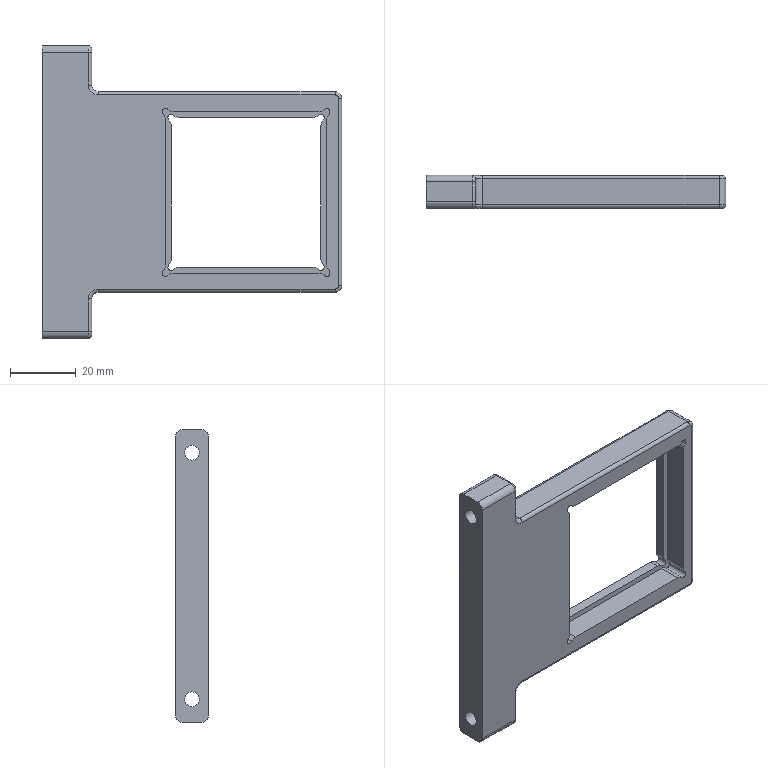NC program | NX | posted by the shop | part box 91 x 10 x 89 mm
Lines 7061 to 8910 of 16928, first 1495 of 1850 lines:
N4 T11 M06
(D4-J  D=4. R=0. H=11 ce=0.00 di=0.01)
G00 G90 G54 X-24.947 Y-33.1 M03 S9000
G43 H11 Z20.
M08
Z-.571
G01 X-24.948 Y-33.094 Z-.656 F2000.
X-24.951 Y-33.074 Z-.734
X-24.956 Y-33.045 Z-.804
X-24.964 Y-33.006 Z-.867
X-24.975 Y-32.961 Z-.922
X-24.989 Y-32.91 Z-.971
X-25.006 Y-32.856 Z-1.014
X-25.027 Y-32.8 Z-1.051
X-25.051 Y-32.744 Z-1.082
X-25.08 Y-32.69 Z-1.107
X-25.112 Y-32.639 Z-1.128
X-25.149 Y-32.594 Z-1.144
X-25.191 Y-32.555 Z-1.156
X-25.238 Y-32.526 Z-1.164
X-25.29 Y-32.507 Z-1.169
X-25.347 Y-32.5 Z-1.171
X-28.489 F2500.
X-28.5
Y-35.653
X-28.484 Y-35.696
X-28.438 Y-35.718 Z-1.174
X-28.366 Y-35.719 Z-1.178
X-28.271 Y-35.702 Z-1.184
X-28.156 Y-35.669 Z-1.19
X-28.026 Y-35.62 Z-1.198
X-27.882 Y-35.557 Z-1.207
X-27.73 Y-35.483 Z-1.217
X-27.571 Y-35.398 Z-1.227
X-27.41 Y-35.304 Z-1.238
X-27.25 Y-35.203 Z-1.25
X-26.913 Y-34.962 Z-1.276
X-26.597 Y-34.695 Z-1.303
X-26.306 Y-34.403 Z-1.331
X-26.038 Y-34.088 Z-1.358
X-25.797 Y-33.75 Z-1.384
X-25.696 Y-33.59 Z-1.395
X-25.602 Y-33.429 Z-1.406
X-25.517 Y-33.27 Z-1.417
X-25.443 Y-33.118 Z-1.427
X-25.38 Y-32.974 Z-1.436
X-25.331 Y-32.844 Z-1.443
X-25.298 Y-32.729 Z-1.45
X-25.281 Y-32.634 Z-1.456
X-25.282 Y-32.562 Z-1.46
X-25.304 Y-32.516 Z-1.462
X-25.347 Y-32.5 Z-1.463
X-28.489
X-28.5
Y-35.653
X-28.484 Y-35.696 Z-1.464
X-28.438 Y-35.718 Z-1.467
X-28.366 Y-35.719 Z-1.471
X-28.271 Y-35.702 Z-1.476
X-28.156 Y-35.669 Z-1.483
X-28.026 Y-35.62 Z-1.491
X-27.882 Y-35.557 Z-1.5
X-27.73 Y-35.483 Z-1.51
X-27.571 Y-35.398 Z-1.52
X-27.41 Y-35.304 Z-1.531
X-27.25 Y-35.203 Z-1.542
X-26.913 Y-34.962 Z-1.569
X-26.597 Y-34.695 Z-1.596
X-26.306 Y-34.403 Z-1.623
X-26.038 Y-34.088 Z-1.65
X-25.797 Y-33.75 Z-1.677
X-25.696 Y-33.59 Z-1.688
X-25.602 Y-33.429 Z-1.699
X-25.517 Y-33.27 Z-1.71
X-25.443 Y-33.118 Z-1.719
X-25.38 Y-32.974 Z-1.728
X-25.331 Y-32.844 Z-1.736
X-25.298 Y-32.729 Z-1.743
X-25.281 Y-32.634 Z-1.748
X-25.282 Y-32.562 Z-1.752
X-25.304 Y-32.516 Z-1.755
X-25.347 Y-32.5 Z-1.756
X-28.489
X-28.5
Y-35.653
X-28.484 Y-35.696 Z-1.757
X-28.438 Y-35.718 Z-1.759
X-28.366 Y-35.719 Z-1.763
X-28.271 Y-35.702 Z-1.769
X-28.156 Y-35.669 Z-1.776
X-28.026 Y-35.62 Z-1.784
X-27.882 Y-35.557 Z-1.792
X-27.73 Y-35.483 Z-1.802
X-27.571 Y-35.398 Z-1.813
X-27.41 Y-35.304 Z-1.824
X-27.25 Y-35.203 Z-1.835
X-26.913 Y-34.962 Z-1.861
X-26.597 Y-34.695 Z-1.889
X-26.306 Y-34.403 Z-1.916
X-26.038 Y-34.088 Z-1.943
X-25.797 Y-33.75 Z-1.969
X-25.696 Y-33.59 Z-1.981
X-25.602 Y-33.429 Z-1.992
X-25.517 Y-33.27 Z-2.002
X-25.443 Y-33.118 Z-2.012
X-25.38 Y-32.974 Z-2.021
X-25.331 Y-32.844 Z-2.029
X-25.298 Y-32.729 Z-2.035
X-25.281 Y-32.634 Z-2.041
X-25.282 Y-32.562 Z-2.045
X-25.304 Y-32.516 Z-2.048
X-25.347 Y-32.5 Z-2.049
X-28.489
X-28.5
Y-35.653
X-28.484 Y-35.696
X-28.438 Y-35.718 Z-2.052
X-28.366 Y-35.719 Z-2.056
X-28.271 Y-35.702 Z-2.062
X-28.156 Y-35.669 Z-2.068
X-28.026 Y-35.62 Z-2.076
X-27.882 Y-35.557 Z-2.085
X-27.73 Y-35.483 Z-2.095
X-27.571 Y-35.398 Z-2.105
X-27.41 Y-35.304 Z-2.116
X-27.25 Y-35.203 Z-2.128
X-26.913 Y-34.962 Z-2.154
X-26.597 Y-34.695 Z-2.181
X-26.306 Y-34.403 Z-2.209
X-26.038 Y-34.088 Z-2.236
X-25.797 Y-33.75 Z-2.262
X-25.696 Y-33.59 Z-2.273
X-25.602 Y-33.429 Z-2.284
X-25.517 Y-33.27 Z-2.295
X-25.443 Y-33.118 Z-2.305
X-25.38 Y-32.974 Z-2.313
X-25.331 Y-32.844 Z-2.321
X-25.298 Y-32.729 Z-2.328
X-25.281 Y-32.634 Z-2.334
X-25.282 Y-32.562 Z-2.338
X-25.304 Y-32.516 Z-2.34
X-25.347 Y-32.5 Z-2.341
X-28.489
X-28.5
Y-35.653
X-28.484 Y-35.696 Z-2.342
X-28.438 Y-35.718 Z-2.345
X-28.366 Y-35.719 Z-2.349
X-28.271 Y-35.702 Z-2.354
X-28.156 Y-35.669 Z-2.361
X-28.026 Y-35.62 Z-2.369
X-27.882 Y-35.557 Z-2.378
X-27.73 Y-35.483 Z-2.387
X-27.571 Y-35.398 Z-2.398
X-27.41 Y-35.304 Z-2.409
X-27.25 Y-35.203 Z-2.42
X-26.913 Y-34.962 Z-2.447
X-26.597 Y-34.695 Z-2.474
X-26.306 Y-34.403 Z-2.501
X-26.038 Y-34.088 Z-2.528
X-25.797 Y-33.75 Z-2.555
X-25.696 Y-33.59 Z-2.566
X-25.602 Y-33.429 Z-2.577
X-25.517 Y-33.27 Z-2.588
X-25.443 Y-33.118 Z-2.597
X-25.38 Y-32.974 Z-2.606
X-25.331 Y-32.844 Z-2.614
X-25.298 Y-32.729 Z-2.621
X-25.281 Y-32.634 Z-2.626
X-25.282 Y-32.562 Z-2.63
X-25.304 Y-32.516 Z-2.633
X-25.347 Y-32.5 Z-2.634
X-28.489
X-28.5
Y-35.653
X-28.484 Y-35.696 Z-2.635
X-28.438 Y-35.718 Z-2.637
X-28.366 Y-35.719 Z-2.641
X-28.271 Y-35.702 Z-2.647
X-28.156 Y-35.669 Z-2.654
X-28.026 Y-35.62 Z-2.662
X-27.882 Y-35.557 Z-2.67
X-27.73 Y-35.483 Z-2.68
X-27.571 Y-35.398 Z-2.691
X-27.41 Y-35.304 Z-2.702
X-27.25 Y-35.203 Z-2.713
X-26.913 Y-34.962 Z-2.739
X-26.597 Y-34.695 Z-2.766
X-26.306 Y-34.403 Z-2.794
X-26.038 Y-34.088 Z-2.821
X-25.797 Y-33.75 Z-2.847
X-25.696 Y-33.59 Z-2.859
X-25.602 Y-33.429 Z-2.87
X-25.517 Y-33.27 Z-2.88
X-25.443 Y-33.118 Z-2.89
X-25.38 Y-32.974 Z-2.899
X-25.331 Y-32.844 Z-2.907
X-25.298 Y-32.729 Z-2.913
X-25.281 Y-32.634 Z-2.919
X-25.282 Y-32.562 Z-2.923
X-25.304 Y-32.516 Z-2.926
X-25.347 Y-32.5
X-28.489
X-28.5
Y-35.653
X-28.484 Y-35.696 Z-2.927
X-28.438 Y-35.718 Z-2.93
X-28.366 Y-35.719 Z-2.934
X-28.271 Y-35.702 Z-2.94
X-28.156 Y-35.669 Z-2.946
X-28.026 Y-35.62 Z-2.954
X-27.882 Y-35.557 Z-2.963
X-27.73 Y-35.483 Z-2.973
X-27.571 Y-35.398 Z-2.983
X-27.41 Y-35.304 Z-2.994
X-27.25 Y-35.203 Z-3.006
X-26.913 Y-34.962 Z-3.032
X-26.597 Y-34.695 Z-3.059
X-26.306 Y-34.403 Z-3.087
X-26.038 Y-34.088 Z-3.114
X-25.797 Y-33.75 Z-3.14
X-25.696 Y-33.59 Z-3.151
X-25.602 Y-33.429 Z-3.162
X-25.517 Y-33.27 Z-3.173
X-25.443 Y-33.118 Z-3.183
X-25.38 Y-32.974 Z-3.191
X-25.331 Y-32.844 Z-3.199
X-25.298 Y-32.729 Z-3.206
X-25.281 Y-32.634 Z-3.212
X-25.282 Y-32.562 Z-3.216
X-25.304 Y-32.516 Z-3.218
X-25.347 Y-32.5 Z-3.219
X-28.489
X-28.5
Y-35.653
X-28.484 Y-35.696 Z-3.22
X-28.438 Y-35.718 Z-3.223
X-28.366 Y-35.719 Z-3.227
X-28.271 Y-35.702 Z-3.232
X-28.156 Y-35.669 Z-3.239
X-28.026 Y-35.62 Z-3.247
X-27.882 Y-35.557 Z-3.256
X-27.73 Y-35.483 Z-3.265
X-27.571 Y-35.398 Z-3.276
X-27.41 Y-35.304 Z-3.287
X-27.25 Y-35.203 Z-3.298
X-26.913 Y-34.962 Z-3.325
X-26.597 Y-34.695 Z-3.352
X-26.306 Y-34.403 Z-3.379
X-26.038 Y-34.088 Z-3.406
X-25.797 Y-33.75 Z-3.433
X-25.696 Y-33.59 Z-3.444
X-25.602 Y-33.429 Z-3.455
X-25.517 Y-33.27 Z-3.465
X-25.443 Y-33.118 Z-3.475
X-25.38 Y-32.974 Z-3.484
X-25.331 Y-32.844 Z-3.492
X-25.298 Y-32.729 Z-3.499
X-25.281 Y-32.634 Z-3.504
X-25.282 Y-32.562 Z-3.508
X-25.304 Y-32.516 Z-3.511
X-25.347 Y-32.5 Z-3.512
X-28.489
X-28.5
Y-35.653
X-28.484 Y-35.696 Z-3.513
X-28.438 Y-35.718 Z-3.515
X-28.366 Y-35.719 Z-3.519
X-28.271 Y-35.702 Z-3.525
X-28.156 Y-35.669 Z-3.532
X-28.026 Y-35.62 Z-3.539
X-27.882 Y-35.557 Z-3.548
X-27.73 Y-35.483 Z-3.558
X-27.571 Y-35.398 Z-3.569
X-27.41 Y-35.304 Z-3.58
X-27.25 Y-35.203 Z-3.591
X-26.913 Y-34.962 Z-3.617
X-26.597 Y-34.695 Z-3.644
X-26.306 Y-34.403 Z-3.672
X-26.038 Y-34.088 Z-3.699
X-25.797 Y-33.75 Z-3.725
X-25.696 Y-33.59 Z-3.737
X-25.602 Y-33.429 Z-3.748
X-25.517 Y-33.27 Z-3.758
X-25.443 Y-33.118 Z-3.768
X-25.38 Y-32.974 Z-3.777
X-25.331 Y-32.844 Z-3.785
X-25.298 Y-32.729 Z-3.791
X-25.281 Y-32.634 Z-3.797
X-25.282 Y-32.562 Z-3.801
X-25.304 Y-32.516 Z-3.804
X-25.347 Y-32.5
X-28.489
X-28.5
Y-35.653
X-28.484 Y-35.696 Z-3.805
X-28.438 Y-35.718 Z-3.808
X-28.366 Y-35.719 Z-3.812
X-28.271 Y-35.702 Z-3.817
X-28.156 Y-35.669 Z-3.824
X-28.026 Y-35.62 Z-3.832
X-27.882 Y-35.557 Z-3.841
X-27.73 Y-35.483 Z-3.851
X-27.571 Y-35.398 Z-3.861
X-27.41 Y-35.304 Z-3.872
X-27.25 Y-35.203 Z-3.884
X-26.913 Y-34.962 Z-3.91
X-26.597 Y-34.695 Z-3.937
X-26.306 Y-34.403 Z-3.964
X-26.038 Y-34.088 Z-3.992
X-25.797 Y-33.75 Z-4.018
X-25.696 Y-33.59 Z-4.029
X-25.602 Y-33.429 Z-4.04
X-25.517 Y-33.27 Z-4.051
X-25.443 Y-33.118 Z-4.06
X-25.38 Y-32.974 Z-4.069
X-25.331 Y-32.844 Z-4.077
X-25.298 Y-32.729 Z-4.084
X-25.281 Y-32.634 Z-4.09
X-25.282 Y-32.562 Z-4.094
X-25.304 Y-32.516 Z-4.096
X-25.347 Y-32.5 Z-4.097
X-28.489
X-28.5
Y-35.653
X-28.484 Y-35.696 Z-4.098
X-28.438 Y-35.718 Z-4.101
X-28.366 Y-35.719 Z-4.105
X-28.271 Y-35.702 Z-4.11
X-28.156 Y-35.669 Z-4.117
X-28.026 Y-35.62 Z-4.125
X-27.882 Y-35.557 Z-4.134
X-27.73 Y-35.483 Z-4.143
X-27.571 Y-35.398 Z-4.154
X-27.41 Y-35.304 Z-4.165
X-27.25 Y-35.203 Z-4.176
X-26.913 Y-34.962 Z-4.203
X-26.597 Y-34.695 Z-4.23
X-26.306 Y-34.403 Z-4.257
X-26.038 Y-34.088 Z-4.284
X-25.797 Y-33.75 Z-4.31
X-25.696 Y-33.59 Z-4.322
X-25.602 Y-33.429 Z-4.333
X-25.517 Y-33.27 Z-4.343
X-25.443 Y-33.118 Z-4.353
X-25.38 Y-32.974 Z-4.362
X-25.331 Y-32.844 Z-4.37
X-25.298 Y-32.729 Z-4.377
X-25.281 Y-32.634 Z-4.382
X-25.282 Y-32.562 Z-4.386
X-25.304 Y-32.516 Z-4.389
X-25.347 Y-32.5 Z-4.39
X-28.489
X-28.5
Y-35.653
X-28.484 Y-35.696 Z-4.391
X-28.438 Y-35.718 Z-4.393
X-28.366 Y-35.719 Z-4.397
X-28.271 Y-35.702 Z-4.403
X-28.156 Y-35.669 Z-4.41
X-28.026 Y-35.62 Z-4.417
X-27.882 Y-35.557 Z-4.426
X-27.73 Y-35.483 Z-4.436
X-27.571 Y-35.398 Z-4.446
X-27.41 Y-35.304 Z-4.458
X-27.25 Y-35.203 Z-4.469
X-26.913 Y-34.962 Z-4.495
X-26.597 Y-34.695 Z-4.522
X-26.306 Y-34.403 Z-4.55
X-26.038 Y-34.088 Z-4.577
X-25.797 Y-33.75 Z-4.603
X-25.696 Y-33.59 Z-4.615
X-25.602 Y-33.429 Z-4.626
X-25.517 Y-33.27 Z-4.636
X-25.443 Y-33.118 Z-4.646
X-25.38 Y-32.974 Z-4.655
X-25.331 Y-32.844 Z-4.663
X-25.298 Y-32.729 Z-4.669
X-25.281 Y-32.634 Z-4.675
X-25.282 Y-32.562 Z-4.679
X-25.304 Y-32.516 Z-4.681
X-25.347 Y-32.5 Z-4.682
X-28.489
X-28.5
Y-35.653
X-28.484 Y-35.696 Z-4.683
X-28.438 Y-35.718 Z-4.686
X-28.366 Y-35.719 Z-4.69
X-28.271 Y-35.702 Z-4.695
X-28.156 Y-35.669 Z-4.702
X-28.026 Y-35.62 Z-4.71
X-27.882 Y-35.557 Z-4.719
X-27.73 Y-35.483 Z-4.729
X-27.571 Y-35.398 Z-4.739
X-27.41 Y-35.304 Z-4.75
X-27.25 Y-35.203 Z-4.762
X-26.913 Y-34.962 Z-4.788
X-26.597 Y-34.695 Z-4.815
X-26.306 Y-34.403 Z-4.842
X-26.038 Y-34.088 Z-4.87
X-25.797 Y-33.75 Z-4.896
X-25.696 Y-33.59 Z-4.907
X-25.602 Y-33.429 Z-4.918
X-25.517 Y-33.27 Z-4.929
X-25.443 Y-33.118 Z-4.938
X-25.38 Y-32.974 Z-4.947
X-25.331 Y-32.844 Z-4.955
X-25.298 Y-32.729 Z-4.962
X-25.281 Y-32.634 Z-4.967
X-25.282 Y-32.562 Z-4.972
X-25.304 Y-32.516 Z-4.974
X-25.347 Y-32.5 Z-4.975
X-28.489
X-28.5
Y-35.653
X-28.484 Y-35.696 Z-4.976
X-28.438 Y-35.718 Z-4.978
X-28.366 Y-35.719 Z-4.983
X-28.271 Y-35.702 Z-4.988
X-28.156 Y-35.669 Z-4.995
X-28.026 Y-35.62 Z-5.003
X-27.882 Y-35.557 Z-5.012
X-27.73 Y-35.483 Z-5.021
X-27.571 Y-35.398 Z-5.032
X-27.41 Y-35.304 Z-5.043
X-27.25 Y-35.203 Z-5.054
X-26.913 Y-34.962 Z-5.081
X-26.597 Y-34.695 Z-5.108
X-26.306 Y-34.403 Z-5.135
X-26.038 Y-34.088 Z-5.162
X-25.797 Y-33.75 Z-5.188
X-25.696 Y-33.59 Z-5.2
X-25.602 Y-33.429 Z-5.211
X-25.517 Y-33.27 Z-5.221
X-25.443 Y-33.118 Z-5.231
X-25.38 Y-32.974 Z-5.24
X-25.331 Y-32.844 Z-5.248
X-25.298 Y-32.729 Z-5.255
X-25.281 Y-32.634 Z-5.26
X-25.282 Y-32.562 Z-5.264
X-25.304 Y-32.516 Z-5.267
X-25.347 Y-32.5 Z-5.268
X-28.489
X-28.5
Y-35.653
X-28.484 Y-35.696 Z-5.269
X-28.438 Y-35.718 Z-5.271
X-28.366 Y-35.719 Z-5.275
X-28.271 Y-35.702 Z-5.281
X-28.156 Y-35.669 Z-5.287
X-28.026 Y-35.62 Z-5.295
X-27.882 Y-35.557 Z-5.304
X-27.73 Y-35.483 Z-5.314
X-27.571 Y-35.398 Z-5.324
X-27.41 Y-35.304 Z-5.335
X-27.25 Y-35.203 Z-5.347
X-26.913 Y-34.962 Z-5.373
X-26.597 Y-34.695 Z-5.4
X-26.306 Y-34.403 Z-5.428
X-26.038 Y-34.088 Z-5.455
X-25.797 Y-33.75 Z-5.481
X-25.696 Y-33.59 Z-5.493
X-25.602 Y-33.429 Z-5.504
X-25.517 Y-33.27 Z-5.514
X-25.443 Y-33.118 Z-5.524
X-25.38 Y-32.974 Z-5.533
X-25.331 Y-32.844 Z-5.54
X-25.298 Y-32.729 Z-5.547
X-25.281 Y-32.634 Z-5.553
X-25.282 Y-32.562 Z-5.557
X-25.304 Y-32.516 Z-5.559
X-25.347 Y-32.5 Z-5.56
X-28.489
X-28.5
Y-35.653
X-28.484 Y-35.696 Z-5.561
X-28.438 Y-35.718 Z-5.564
X-28.366 Y-35.719 Z-5.568
X-28.271 Y-35.702 Z-5.573
X-28.156 Y-35.669 Z-5.58
X-28.026 Y-35.62 Z-5.588
X-27.882 Y-35.557 Z-5.597
X-27.73 Y-35.483 Z-5.607
X-27.571 Y-35.398 Z-5.617
X-27.41 Y-35.304 Z-5.628
X-27.25 Y-35.203 Z-5.64
X-26.913 Y-34.962 Z-5.666
X-26.597 Y-34.695 Z-5.693
X-26.306 Y-34.403 Z-5.72
X-26.038 Y-34.088 Z-5.747
X-25.797 Y-33.75 Z-5.774
X-25.696 Y-33.59 Z-5.785
X-25.602 Y-33.429 Z-5.796
X-25.517 Y-33.27 Z-5.807
X-25.443 Y-33.118 Z-5.816
X-25.38 Y-32.974 Z-5.825
X-25.331 Y-32.844 Z-5.833
X-25.298 Y-32.729 Z-5.84
X-25.281 Y-32.634 Z-5.845
X-25.282 Y-32.562 Z-5.849
X-25.304 Y-32.516 Z-5.852
X-25.347 Y-32.5 Z-5.853
X-28.489
X-28.5
Y-35.653
X-28.484 Y-35.696 Z-5.854
X-28.438 Y-35.718 Z-5.856
X-28.366 Y-35.719 Z-5.86
X-28.271 Y-35.702 Z-5.866
X-28.156 Y-35.669 Z-5.873
X-28.026 Y-35.62 Z-5.881
X-27.882 Y-35.557 Z-5.89
X-27.73 Y-35.483 Z-5.899
X-27.571 Y-35.398 Z-5.91
X-27.41 Y-35.304 Z-5.921
X-27.25 Y-35.203 Z-5.932
X-26.913 Y-34.962 Z-5.958
X-26.597 Y-34.695 Z-5.986
X-26.306 Y-34.403 Z-6.013
X-26.038 Y-34.088 Z-6.04
X-25.797 Y-33.75 Z-6.066
X-25.696 Y-33.59 Z-6.078
X-25.602 Y-33.429 Z-6.089
X-25.517 Y-33.27 Z-6.099
X-25.443 Y-33.118 Z-6.109
X-25.38 Y-32.974 Z-6.118
X-25.331 Y-32.844 Z-6.126
X-25.298 Y-32.729 Z-6.133
X-25.281 Y-32.634 Z-6.138
X-25.282 Y-32.562 Z-6.142
X-25.304 Y-32.516 Z-6.145
X-25.347 Y-32.5 Z-6.146
X-28.489
X-28.5
Y-35.653
X-28.484 Y-35.696
X-28.438 Y-35.718 Z-6.149
X-28.366 Y-35.719 Z-6.153
X-28.271 Y-35.702 Z-6.159
X-28.156 Y-35.669 Z-6.165
X-28.026 Y-35.62 Z-6.173
X-27.882 Y-35.557 Z-6.182
X-27.73 Y-35.483 Z-6.192
X-27.571 Y-35.398 Z-6.202
X-27.41 Y-35.304 Z-6.213
X-27.25 Y-35.203 Z-6.225
X-26.913 Y-34.962 Z-6.251
X-26.597 Y-34.695 Z-6.278
X-26.306 Y-34.403 Z-6.306
X-26.038 Y-34.088 Z-6.333
X-25.797 Y-33.75 Z-6.359
X-25.696 Y-33.59 Z-6.37
X-25.602 Y-33.429 Z-6.381
X-25.517 Y-33.27 Z-6.392
X-25.443 Y-33.118 Z-6.402
X-25.38 Y-32.974 Z-6.411
X-25.331 Y-32.844 Z-6.418
X-25.298 Y-32.729 Z-6.425
X-25.281 Y-32.634 Z-6.431
X-25.282 Y-32.562 Z-6.435
X-25.304 Y-32.516 Z-6.437
X-25.347 Y-32.5 Z-6.438
X-28.489
X-28.5
Y-35.653
X-28.484 Y-35.696 Z-6.439
X-28.438 Y-35.718 Z-6.442
X-28.366 Y-35.719 Z-6.446
X-28.271 Y-35.702 Z-6.451
X-28.156 Y-35.669 Z-6.458
X-28.026 Y-35.62 Z-6.466
X-27.882 Y-35.557 Z-6.475
X-27.73 Y-35.483 Z-6.485
X-27.571 Y-35.398 Z-6.495
X-27.41 Y-35.304 Z-6.506
X-27.25 Y-35.203 Z-6.517
X-26.913 Y-34.962 Z-6.544
X-26.597 Y-34.695 Z-6.571
X-26.306 Y-34.403 Z-6.598
X-26.038 Y-34.088 Z-6.625
X-25.797 Y-33.75 Z-6.652
X-25.696 Y-33.59 Z-6.663
X-25.602 Y-33.429 Z-6.674
X-25.517 Y-33.27 Z-6.685
X-25.443 Y-33.118 Z-6.694
X-25.38 Y-32.974 Z-6.703
X-25.331 Y-32.844 Z-6.711
X-25.298 Y-32.729 Z-6.718
X-25.281 Y-32.634 Z-6.723
X-25.282 Y-32.562 Z-6.727
X-25.304 Y-32.516 Z-6.73
X-25.347 Y-32.5 Z-6.731
X-28.489
X-28.5
Y-35.653
X-28.484 Y-35.696 Z-6.732
X-28.438 Y-35.718 Z-6.734
X-28.366 Y-35.719 Z-6.738
X-28.271 Y-35.702 Z-6.744
X-28.156 Y-35.669 Z-6.751
X-28.026 Y-35.62 Z-6.759
X-27.882 Y-35.557 Z-6.767
X-27.73 Y-35.483 Z-6.777
X-27.571 Y-35.398 Z-6.788
X-27.41 Y-35.304 Z-6.799
X-27.25 Y-35.203 Z-6.81
X-26.913 Y-34.962 Z-6.836
X-26.597 Y-34.695 Z-6.864
X-26.306 Y-34.403 Z-6.891
X-26.038 Y-34.088 Z-6.918
X-25.797 Y-33.75 Z-6.944
X-25.696 Y-33.59 Z-6.956
X-25.602 Y-33.429 Z-6.967
X-25.517 Y-33.27 Z-6.977
X-25.443 Y-33.118 Z-6.987
X-25.38 Y-32.974 Z-6.996
X-25.331 Y-32.844 Z-7.004
X-25.298 Y-32.729 Z-7.01
X-25.281 Y-32.634 Z-7.016
X-25.282 Y-32.562 Z-7.02
X-25.304 Y-32.516 Z-7.023
X-25.347 Y-32.5 Z-7.024
X-28.489
X-28.5
Y-35.653
X-28.484 Y-35.696
X-28.438 Y-35.718 Z-7.027
X-28.366 Y-35.719 Z-7.031
X-28.271 Y-35.702 Z-7.037
X-28.156 Y-35.669 Z-7.043
X-28.026 Y-35.62 Z-7.051
X-27.882 Y-35.557 Z-7.06
X-27.73 Y-35.483 Z-7.07
X-27.571 Y-35.398 Z-7.08
X-27.41 Y-35.304 Z-7.091
X-27.25 Y-35.203 Z-7.103
X-26.913 Y-34.962 Z-7.129
X-26.597 Y-34.695 Z-7.156
X-26.306 Y-34.403 Z-7.184
X-26.038 Y-34.088 Z-7.211
X-25.797 Y-33.75 Z-7.237
X-25.696 Y-33.59 Z-7.248
X-25.602 Y-33.429 Z-7.259
X-25.517 Y-33.27 Z-7.27
X-25.443 Y-33.118 Z-7.28
X-25.38 Y-32.974 Z-7.288
X-25.331 Y-32.844 Z-7.296
X-25.298 Y-32.729 Z-7.303
X-25.281 Y-32.634 Z-7.309
X-25.282 Y-32.562 Z-7.313
X-25.304 Y-32.516 Z-7.315
X-25.347 Y-32.5 Z-7.316
X-28.489
X-28.5
Y-35.653
X-28.484 Y-35.696 Z-7.317
X-28.438 Y-35.718 Z-7.32
X-28.366 Y-35.719 Z-7.324
X-28.271 Y-35.702 Z-7.329
X-28.156 Y-35.669 Z-7.336
X-28.026 Y-35.62 Z-7.344
X-27.882 Y-35.557 Z-7.353
X-27.73 Y-35.483 Z-7.362
X-27.571 Y-35.398 Z-7.373
X-27.41 Y-35.304 Z-7.384
X-27.25 Y-35.203 Z-7.395
X-26.913 Y-34.962 Z-7.422
X-26.597 Y-34.695 Z-7.449
X-26.306 Y-34.403 Z-7.476
X-26.038 Y-34.088 Z-7.503
X-25.797 Y-33.75 Z-7.53
X-25.696 Y-33.59 Z-7.541
X-25.602 Y-33.429 Z-7.552
X-25.517 Y-33.27 Z-7.563
X-25.443 Y-33.118 Z-7.572
X-25.38 Y-32.974 Z-7.581
X-25.331 Y-32.844 Z-7.589
X-25.298 Y-32.729 Z-7.596
X-25.281 Y-32.634 Z-7.601
X-25.282 Y-32.562 Z-7.605
X-25.304 Y-32.516 Z-7.608
X-25.347 Y-32.5 Z-7.609
X-28.489
X-28.5
Y-35.653
X-28.484 Y-35.696 Z-7.61
X-28.438 Y-35.718 Z-7.612
X-28.366 Y-35.719 Z-7.616
X-28.271 Y-35.702 Z-7.622
X-28.156 Y-35.669 Z-7.629
X-28.026 Y-35.62 Z-7.637
X-27.882 Y-35.557 Z-7.645
X-27.73 Y-35.483 Z-7.655
X-27.571 Y-35.398 Z-7.666
X-27.41 Y-35.304 Z-7.677
X-27.25 Y-35.203 Z-7.688
X-26.913 Y-34.962 Z-7.714
X-26.597 Y-34.695 Z-7.741
X-26.306 Y-34.403 Z-7.769
X-26.038 Y-34.088 Z-7.796
X-25.797 Y-33.75 Z-7.822
X-25.696 Y-33.59 Z-7.834
X-25.602 Y-33.429 Z-7.845
X-25.517 Y-33.27 Z-7.855
X-25.443 Y-33.118 Z-7.865
X-25.38 Y-32.974 Z-7.874
X-25.331 Y-32.844 Z-7.882
X-25.298 Y-32.729 Z-7.888
X-25.281 Y-32.634 Z-7.894
X-25.282 Y-32.562 Z-7.898
X-25.304 Y-32.516 Z-7.901
X-25.347 Y-32.5
X-28.489
X-28.5
Y-35.653
X-28.484 Y-35.696 Z-7.902
X-28.438 Y-35.718 Z-7.905
X-28.366 Y-35.719 Z-7.909
X-28.271 Y-35.702 Z-7.915
X-28.156 Y-35.669 Z-7.921
X-28.026 Y-35.62 Z-7.929
X-27.882 Y-35.557 Z-7.938
X-27.73 Y-35.483 Z-7.948
X-27.571 Y-35.398 Z-7.958
X-27.41 Y-35.304 Z-7.969
X-27.25 Y-35.203 Z-7.981
X-26.913 Y-34.962 Z-8.007
X-26.597 Y-34.695 Z-8.034
X-26.306 Y-34.403 Z-8.062
X-26.038 Y-34.088 Z-8.089
X-25.797 Y-33.75 Z-8.115
X-25.696 Y-33.59 Z-8.126
X-25.602 Y-33.429 Z-8.137
X-25.517 Y-33.27 Z-8.148
X-25.443 Y-33.118 Z-8.158
X-25.38 Y-32.974 Z-8.166
X-25.331 Y-32.844 Z-8.174
X-25.298 Y-32.729 Z-8.181
X-25.281 Y-32.634 Z-8.187
X-25.282 Y-32.562 Z-8.191
X-25.304 Y-32.516 Z-8.193
X-25.347 Y-32.5 Z-8.194
X-28.489
X-28.5
Y-35.653
X-28.484 Y-35.696 Z-8.195
X-28.438 Y-35.718 Z-8.198
X-28.366 Y-35.719 Z-8.202
X-28.271 Y-35.702 Z-8.207
X-28.156 Y-35.669 Z-8.214
X-28.026 Y-35.62 Z-8.222
X-27.882 Y-35.557 Z-8.231
X-27.73 Y-35.483 Z-8.24
X-27.571 Y-35.398 Z-8.251
X-27.41 Y-35.304 Z-8.262
X-27.25 Y-35.203 Z-8.273
X-26.913 Y-34.962 Z-8.3
X-26.597 Y-34.695 Z-8.327
X-26.306 Y-34.403 Z-8.354
X-26.038 Y-34.088 Z-8.381
X-25.797 Y-33.75 Z-8.408
X-25.696 Y-33.59 Z-8.419
X-25.602 Y-33.429 Z-8.43
X-25.517 Y-33.27 Z-8.44
X-25.443 Y-33.118 Z-8.45
X-25.38 Y-32.974 Z-8.459
X-25.331 Y-32.844 Z-8.467
X-25.298 Y-32.729 Z-8.474
X-25.281 Y-32.634 Z-8.479
X-25.282 Y-32.562 Z-8.483
X-25.304 Y-32.516 Z-8.486
X-25.347 Y-32.5 Z-8.487
X-28.489
X-28.5
Y-35.653
X-28.484 Y-35.696 Z-8.488
X-28.438 Y-35.718 Z-8.49
X-28.366 Y-35.719 Z-8.494
X-28.271 Y-35.702 Z-8.5
X-28.156 Y-35.669 Z-8.507
X-28.026 Y-35.62 Z-8.514
X-27.882 Y-35.557 Z-8.523
X-27.73 Y-35.483 Z-8.533
X-27.571 Y-35.398 Z-8.544
X-27.41 Y-35.304 Z-8.555
X-27.25 Y-35.203 Z-8.566
X-26.913 Y-34.962 Z-8.592
X-26.597 Y-34.695 Z-8.619
X-26.306 Y-34.403 Z-8.647
X-26.038 Y-34.088 Z-8.674
X-25.797 Y-33.75 Z-8.7
X-25.696 Y-33.59 Z-8.712
X-25.602 Y-33.429 Z-8.723
X-25.517 Y-33.27 Z-8.733
X-25.443 Y-33.118 Z-8.743
X-25.38 Y-32.974 Z-8.752
X-25.331 Y-32.844 Z-8.76
X-25.298 Y-32.729 Z-8.766
X-25.281 Y-32.634 Z-8.772
X-25.282 Y-32.562 Z-8.776
X-25.304 Y-32.516 Z-8.779
X-25.347 Y-32.5
X-28.489
X-28.5
Y-35.653
X-28.484 Y-35.696 Z-8.78
X-28.438 Y-35.718 Z-8.783
X-28.366 Y-35.719 Z-8.787
X-28.271 Y-35.702 Z-8.792
X-28.156 Y-35.669 Z-8.799
X-28.025 Y-35.62 Z-8.807
X-27.882 Y-35.557 Z-8.816
X-27.729 Y-35.483 Z-8.826
X-27.57 Y-35.398 Z-8.836
X-27.409 Y-35.304 Z-8.847
X-27.249 Y-35.203 Z-8.859
X-26.911 Y-34.962 Z-8.885
X-26.596 Y-34.695 Z-8.912
X-26.303 Y-34.403 Z-8.939
X-26.036 Y-34.088 Z-8.967
X-25.794 Y-33.75 Z-8.993
X-25.693 Y-33.59 Z-9.004
X-25.599 Y-33.429 Z-9.015
X-25.514 Y-33.27 Z-9.026
X-25.44 Y-33.118 Z-9.035
X-25.377 Y-32.974 Z-9.044
X-25.328 Y-32.844 Z-9.052
X-25.294 Y-32.729 Z-9.059
X-25.277 Y-32.634 Z-9.065
X-25.278 Y-32.562 Z-9.069
X-25.3 Y-32.516 Z-9.071
X-25.343 Y-32.5 Z-9.072
X-28.5
Y-35.655
X-28.484 Y-35.698 Z-9.073
X-28.438 Y-35.72 Z-9.076
X-28.366 Y-35.721 Z-9.08
X-28.271 Y-35.704 Z-9.085
X-28.156 Y-35.67 Z-9.092
X-28.025 Y-35.621 Z-9.1
X-27.882 Y-35.559 Z-9.109
X-27.729 Y-35.484 Z-9.118
X-27.57 Y-35.399 Z-9.129
X-27.409 Y-35.306 Z-9.14
X-27.249 Y-35.205 Z-9.151
X-26.911 Y-34.963 Z-9.178
X-26.596 Y-34.696 Z-9.205
X-26.303 Y-34.404 Z-9.232
X-26.036 Y-34.088 Z-9.259
X-25.794 Y-33.75 Z-9.285
X-25.693 Y-33.59 Z-9.297
X-25.599 Y-33.429 Z-9.308
X-25.514 Y-33.271 Z-9.318
X-25.44 Y-33.118 Z-9.328
X-25.377 Y-32.975 Z-9.337
X-25.328 Y-32.844 Z-9.345
X-25.294 Y-32.729 Z-9.352
X-25.277 Y-32.634 Z-9.357
X-25.278 Y-32.562 Z-9.361
X-25.3 Y-32.516 Z-9.364
X-25.343 Y-32.5 Z-9.365
X-28.5
Y-35.655
X-28.484 Y-35.698 Z-9.366
X-28.438 Y-35.72 Z-9.368
X-28.366 Y-35.721 Z-9.372
X-28.271 Y-35.704 Z-9.378
X-28.156 Y-35.67 Z-9.385
X-28.025 Y-35.621 Z-9.392
X-27.882 Y-35.559 Z-9.401
X-27.729 Y-35.484 Z-9.411
X-27.57 Y-35.399 Z-9.421
X-27.409 Y-35.306 Z-9.433
X-27.249 Y-35.205 Z-9.444
X-26.911 Y-34.963 Z-9.47
X-26.596 Y-34.696 Z-9.497
X-26.303 Y-34.404 Z-9.525
X-26.036 Y-34.088 Z-9.552
X-25.794 Y-33.75 Z-9.578
X-25.693 Y-33.59 Z-9.59
X-25.599 Y-33.429 Z-9.601
X-25.514 Y-33.271 Z-9.611
X-25.44 Y-33.118 Z-9.621
X-25.377 Y-32.975 Z-9.63
X-25.328 Y-32.844 Z-9.638
X-25.294 Y-32.729 Z-9.644
X-25.277 Y-32.634 Z-9.65
X-25.278 Y-32.562 Z-9.654
X-25.3 Y-32.516 Z-9.656
X-25.343 Y-32.5 Z-9.657
X-28.5
Y-35.655
X-28.484 Y-35.698 Z-9.658
X-28.438 Y-35.72 Z-9.661
X-28.366 Y-35.721 Z-9.665
X-28.271 Y-35.704 Z-9.67
X-28.156 Y-35.67 Z-9.677
X-28.025 Y-35.621 Z-9.685
X-27.882 Y-35.559 Z-9.694
X-27.729 Y-35.484 Z-9.704
X-27.57 Y-35.399 Z-9.714
X-27.409 Y-35.306 Z-9.725
X-27.249 Y-35.205 Z-9.737
X-26.911 Y-34.963 Z-9.763
X-26.596 Y-34.696 Z-9.79
X-26.303 Y-34.404 Z-9.817
X-26.036 Y-34.088 Z-9.845
X-25.794 Y-33.75 Z-9.871
X-25.693 Y-33.59 Z-9.882
X-25.599 Y-33.429 Z-9.893
X-25.514 Y-33.271 Z-9.904
X-25.44 Y-33.118 Z-9.913
X-25.377 Y-32.975 Z-9.922
X-25.328 Y-32.844 Z-9.93
X-25.294 Y-32.729 Z-9.937
X-25.277 Y-32.634 Z-9.942
X-25.278 Y-32.562 Z-9.947
X-25.3 Y-32.516 Z-9.949
X-25.343 Y-32.5 Z-9.95
X-28.5
Y-35.655
X-28.493 Y-35.712 Z-9.949
X-28.474 Y-35.764 Z-9.944
X-28.445 Y-35.811 Z-9.936
X-28.406 Y-35.852 Z-9.924
X-28.361 Y-35.89 Z-9.908
X-28.31 Y-35.922 Z-9.887
X-28.256 Y-35.951 Z-9.861
X-28.2 Y-35.975 Z-9.83
X-28.144 Y-35.996 Z-9.793
X-28.09 Y-36.013 Z-9.751
X-28.039 Y-36.027 Z-9.702
X-27.994 Y-36.037 Z-9.646
X-27.955 Y-36.045 Z-9.584
X-27.926 Y-36.051 Z-9.514
X-27.907 Y-36.054 Z-9.436
X-27.9 Y-36.055 Z-9.35
G00 Z20.
Y36.053
Z-.571
G01 X-27.907 Y36.052 Z-.656 F2000.
X-27.926 Y36.049 Z-.734
X-27.955 Y36.044 Z-.804
X-27.994 Y36.036 Z-.867
X-28.039 Y36.025 Z-.922
X-28.09 Y36.011 Z-.971
X-28.144 Y35.994 Z-1.014
X-28.2 Y35.973 Z-1.051
X-28.256 Y35.949 Z-1.082
X-28.31 Y35.92 Z-1.107
X-28.361 Y35.888 Z-1.128
X-28.406 Y35.851 Z-1.144
X-28.445 Y35.809 Z-1.156
X-28.474 Y35.762 Z-1.164
X-28.493 Y35.71 Z-1.169
X-28.5 Y35.653 Z-1.171
Y32.5 F2500.
X-25.347
X-25.304 Y32.516
X-25.282 Y32.562 Z-1.174
X-25.281 Y32.634 Z-1.178
X-25.298 Y32.729 Z-1.184
X-25.331 Y32.844 Z-1.19
X-25.38 Y32.974 Z-1.198
X-25.443 Y33.118 Z-1.207
X-25.517 Y33.27 Z-1.217
X-25.602 Y33.429 Z-1.227
X-25.696 Y33.59 Z-1.238
X-25.797 Y33.75 Z-1.25
X-26.038 Y34.087 Z-1.276
X-26.306 Y34.403 Z-1.303
X-26.597 Y34.694 Z-1.331
X-26.913 Y34.962 Z-1.358
X-27.25 Y35.203 Z-1.384
X-27.41 Y35.304 Z-1.395
X-27.571 Y35.398 Z-1.406
X-27.73 Y35.483 Z-1.417
X-27.882 Y35.557 Z-1.427
X-28.026 Y35.62 Z-1.436
X-28.156 Y35.669 Z-1.443
X-28.271 Y35.702 Z-1.45
X-28.366 Y35.719 Z-1.456
X-28.438 Y35.718 Z-1.46
X-28.484 Y35.696 Z-1.462
X-28.5 Y35.653 Z-1.463
Y32.5
X-25.347
X-25.304 Y32.516 Z-1.464
X-25.282 Y32.562 Z-1.467
X-25.281 Y32.634 Z-1.471
X-25.298 Y32.729 Z-1.476
X-25.331 Y32.844 Z-1.483
X-25.38 Y32.974 Z-1.491
X-25.443 Y33.118 Z-1.5
X-25.517 Y33.27 Z-1.51
X-25.602 Y33.429 Z-1.52
X-25.696 Y33.59 Z-1.531
X-25.797 Y33.75 Z-1.542
X-26.038 Y34.087 Z-1.569
X-26.306 Y34.403 Z-1.596
X-26.597 Y34.694 Z-1.623
X-26.913 Y34.962 Z-1.65
X-27.25 Y35.203 Z-1.677
X-27.41 Y35.304 Z-1.688
X-27.571 Y35.398 Z-1.699
X-27.73 Y35.483 Z-1.71
X-27.882 Y35.557 Z-1.719
X-28.026 Y35.62 Z-1.728
X-28.156 Y35.669 Z-1.736
X-28.271 Y35.702 Z-1.743
X-28.366 Y35.719 Z-1.748
X-28.438 Y35.718 Z-1.752
X-28.484 Y35.696 Z-1.755
X-28.5 Y35.653 Z-1.756
Y32.5
X-25.347
X-25.304 Y32.516 Z-1.757
X-25.282 Y32.562 Z-1.759
X-25.281 Y32.634 Z-1.763
X-25.298 Y32.729 Z-1.769
X-25.331 Y32.844 Z-1.776
X-25.38 Y32.974 Z-1.784
X-25.443 Y33.118 Z-1.792
X-25.517 Y33.27 Z-1.802
X-25.602 Y33.429 Z-1.813
X-25.696 Y33.59 Z-1.824
X-25.797 Y33.75 Z-1.835
X-26.038 Y34.087 Z-1.861
X-26.306 Y34.403 Z-1.889
X-26.597 Y34.694 Z-1.916
X-26.913 Y34.962 Z-1.943
X-27.25 Y35.203 Z-1.969
X-27.41 Y35.304 Z-1.981
X-27.571 Y35.398 Z-1.992
X-27.73 Y35.483 Z-2.002
X-27.882 Y35.557 Z-2.012
X-28.026 Y35.62 Z-2.021
X-28.156 Y35.669 Z-2.029
X-28.271 Y35.702 Z-2.035
X-28.366 Y35.719 Z-2.041
X-28.438 Y35.718 Z-2.045
X-28.484 Y35.696 Z-2.048
X-28.5 Y35.653 Z-2.049
Y32.5
X-25.347
X-25.304 Y32.516
X-25.282 Y32.562 Z-2.052
X-25.281 Y32.634 Z-2.056
X-25.298 Y32.729 Z-2.062
X-25.331 Y32.844 Z-2.068
X-25.38 Y32.974 Z-2.076
X-25.443 Y33.118 Z-2.085
X-25.517 Y33.27 Z-2.095
X-25.602 Y33.429 Z-2.105
X-25.696 Y33.59 Z-2.116
X-25.797 Y33.75 Z-2.128
X-26.038 Y34.087 Z-2.154
X-26.306 Y34.403 Z-2.181
X-26.597 Y34.694 Z-2.209
X-26.913 Y34.962 Z-2.236
X-27.25 Y35.203 Z-2.262
X-27.41 Y35.304 Z-2.273
X-27.571 Y35.398 Z-2.284
X-27.73 Y35.483 Z-2.295
X-27.882 Y35.557 Z-2.305
X-28.026 Y35.62 Z-2.313
X-28.156 Y35.669 Z-2.321
X-28.271 Y35.702 Z-2.328
X-28.366 Y35.719 Z-2.334
X-28.438 Y35.718 Z-2.338
X-28.484 Y35.696 Z-2.34
X-28.5 Y35.653 Z-2.341
Y32.5
X-25.347
X-25.304 Y32.516 Z-2.342
X-25.282 Y32.562 Z-2.345
X-25.281 Y32.634 Z-2.349
X-25.298 Y32.729 Z-2.354
X-25.331 Y32.844 Z-2.361
X-25.38 Y32.974 Z-2.369
X-25.443 Y33.118 Z-2.378
X-25.517 Y33.27 Z-2.387
X-25.602 Y33.429 Z-2.398
X-25.696 Y33.59 Z-2.409
X-25.797 Y33.75 Z-2.42
X-26.038 Y34.087 Z-2.447
X-26.306 Y34.403 Z-2.474
X-26.597 Y34.694 Z-2.501
X-26.913 Y34.962 Z-2.528
X-27.25 Y35.203 Z-2.555
X-27.41 Y35.304 Z-2.566
X-27.571 Y35.398 Z-2.577
X-27.73 Y35.483 Z-2.588
X-27.882 Y35.557 Z-2.597
X-28.026 Y35.62 Z-2.606
X-28.156 Y35.669 Z-2.614
X-28.271 Y35.702 Z-2.621
X-28.366 Y35.719 Z-2.626
X-28.438 Y35.718 Z-2.63
X-28.484 Y35.696 Z-2.633
X-28.5 Y35.653 Z-2.634
Y32.5
X-25.347
X-25.304 Y32.516 Z-2.635
X-25.282 Y32.562 Z-2.637
X-25.281 Y32.634 Z-2.641
X-25.298 Y32.729 Z-2.647
X-25.331 Y32.844 Z-2.654
X-25.38 Y32.974 Z-2.662
X-25.443 Y33.118 Z-2.67
X-25.517 Y33.27 Z-2.68
X-25.602 Y33.429 Z-2.691
X-25.696 Y33.59 Z-2.702
X-25.797 Y33.75 Z-2.713
X-26.038 Y34.087 Z-2.739
X-26.306 Y34.403 Z-2.766
X-26.597 Y34.694 Z-2.794
X-26.913 Y34.962 Z-2.821
X-27.25 Y35.203 Z-2.847
X-27.41 Y35.304 Z-2.859
X-27.571 Y35.398 Z-2.87
X-27.73 Y35.483 Z-2.88
X-27.882 Y35.557 Z-2.89
X-28.026 Y35.62 Z-2.899
X-28.156 Y35.669 Z-2.907
X-28.271 Y35.702 Z-2.913
X-28.366 Y35.719 Z-2.919
X-28.438 Y35.718 Z-2.923
X-28.484 Y35.696 Z-2.926
X-28.5 Y35.653
Y32.5
X-25.347
X-25.304 Y32.516 Z-2.927
X-25.282 Y32.562 Z-2.93
X-25.281 Y32.634 Z-2.934
X-25.298 Y32.729 Z-2.94
X-25.331 Y32.844 Z-2.946
X-25.38 Y32.974 Z-2.954
X-25.443 Y33.118 Z-2.963
X-25.517 Y33.27 Z-2.973
X-25.602 Y33.429 Z-2.983
X-25.696 Y33.59 Z-2.994
X-25.797 Y33.75 Z-3.006
X-26.038 Y34.087 Z-3.032
X-26.306 Y34.403 Z-3.059
X-26.597 Y34.694 Z-3.087
X-26.913 Y34.962 Z-3.114
X-27.25 Y35.203 Z-3.14
X-27.41 Y35.304 Z-3.151
X-27.571 Y35.398 Z-3.162
X-27.73 Y35.483 Z-3.173
X-27.882 Y35.557 Z-3.183
X-28.026 Y35.62 Z-3.191
X-28.156 Y35.669 Z-3.199
X-28.271 Y35.702 Z-3.206
X-28.366 Y35.719 Z-3.212
X-28.438 Y35.718 Z-3.216
X-28.484 Y35.696 Z-3.218
X-28.5 Y35.653 Z-3.219
Y32.5
X-25.347
X-25.304 Y32.516 Z-3.22
X-25.282 Y32.562 Z-3.223
X-25.281 Y32.634 Z-3.227
X-25.298 Y32.729 Z-3.232
X-25.331 Y32.844 Z-3.239
X-25.38 Y32.974 Z-3.247
X-25.443 Y33.118 Z-3.256
X-25.517 Y33.27 Z-3.265
X-25.602 Y33.429 Z-3.276
X-25.696 Y33.59 Z-3.287
X-25.797 Y33.75 Z-3.298
X-26.038 Y34.087 Z-3.325
X-26.306 Y34.403 Z-3.352
X-26.597 Y34.694 Z-3.379
X-26.913 Y34.962 Z-3.406
X-27.25 Y35.203 Z-3.433
X-27.41 Y35.304 Z-3.444
X-27.571 Y35.398 Z-3.455
X-27.73 Y35.483 Z-3.465
X-27.882 Y35.557 Z-3.475
X-28.026 Y35.62 Z-3.484
X-28.156 Y35.669 Z-3.492
X-28.271 Y35.702 Z-3.499
X-28.366 Y35.719 Z-3.504
X-28.438 Y35.718 Z-3.508
X-28.484 Y35.696 Z-3.511
X-28.5 Y35.653 Z-3.512
Y32.5
X-25.347
X-25.304 Y32.516 Z-3.513
X-25.282 Y32.562 Z-3.515
X-25.281 Y32.634 Z-3.519
X-25.298 Y32.729 Z-3.525
X-25.331 Y32.844 Z-3.532
X-25.38 Y32.974 Z-3.539
X-25.443 Y33.118 Z-3.548
X-25.517 Y33.27 Z-3.558
X-25.602 Y33.429 Z-3.569
X-25.696 Y33.59 Z-3.58
X-25.797 Y33.75 Z-3.591
X-26.038 Y34.087 Z-3.617
X-26.306 Y34.403 Z-3.644
X-26.597 Y34.694 Z-3.672
X-26.913 Y34.962 Z-3.699
X-27.25 Y35.203 Z-3.725
X-27.41 Y35.304 Z-3.737
X-27.571 Y35.398 Z-3.748
X-27.73 Y35.483 Z-3.758
X-27.882 Y35.557 Z-3.768
X-28.026 Y35.62 Z-3.777
X-28.156 Y35.669 Z-3.785
X-28.271 Y35.702 Z-3.791
X-28.366 Y35.719 Z-3.797
X-28.438 Y35.718 Z-3.801
X-28.484 Y35.696 Z-3.804
X-28.5 Y35.653
Y32.5
X-25.347
X-25.304 Y32.516 Z-3.805
X-25.282 Y32.562 Z-3.808
X-25.281 Y32.634 Z-3.812
X-25.298 Y32.729 Z-3.817
X-25.331 Y32.844 Z-3.824
X-25.38 Y32.974 Z-3.832
X-25.443 Y33.118 Z-3.841
X-25.517 Y33.27 Z-3.851
X-25.602 Y33.429 Z-3.861
X-25.696 Y33.59 Z-3.872
X-25.797 Y33.75 Z-3.884
X-26.038 Y34.087 Z-3.91
X-26.306 Y34.403 Z-3.937
X-26.597 Y34.694 Z-3.964
X-26.913 Y34.962 Z-3.992
X-27.25 Y35.203 Z-4.018
X-27.41 Y35.304 Z-4.029
X-27.571 Y35.398 Z-4.04
X-27.73 Y35.483 Z-4.051
X-27.882 Y35.557 Z-4.06
X-28.026 Y35.62 Z-4.069
X-28.156 Y35.669 Z-4.077
X-28.271 Y35.702 Z-4.084
X-28.366 Y35.719 Z-4.09
X-28.438 Y35.718 Z-4.094
X-28.484 Y35.696 Z-4.096
X-28.5 Y35.653 Z-4.097
Y32.5
X-25.347
X-25.304 Y32.516 Z-4.098
X-25.282 Y32.562 Z-4.101
X-25.281 Y32.634 Z-4.105
X-25.298 Y32.729 Z-4.11
X-25.331 Y32.844 Z-4.117
X-25.38 Y32.974 Z-4.125
X-25.443 Y33.118 Z-4.134
X-25.517 Y33.27 Z-4.143
X-25.602 Y33.429 Z-4.154
X-25.696 Y33.59 Z-4.165
X-25.797 Y33.75 Z-4.176
X-26.038 Y34.087 Z-4.203
X-26.306 Y34.403 Z-4.23
X-26.597 Y34.694 Z-4.257
X-26.913 Y34.962 Z-4.284
X-27.25 Y35.203 Z-4.31
X-27.41 Y35.304 Z-4.322
X-27.571 Y35.398 Z-4.333
X-27.73 Y35.483 Z-4.343
X-27.882 Y35.557 Z-4.353
X-28.026 Y35.62 Z-4.362
X-28.156 Y35.669 Z-4.37
X-28.271 Y35.702 Z-4.377
X-28.366 Y35.719 Z-4.382
X-28.438 Y35.718 Z-4.386
X-28.484 Y35.696 Z-4.389
X-28.5 Y35.653 Z-4.39
Y32.5
X-25.347
X-25.304 Y32.516 Z-4.391
X-25.282 Y32.562 Z-4.393
X-25.281 Y32.634 Z-4.397
X-25.298 Y32.729 Z-4.403
X-25.331 Y32.844 Z-4.41
X-25.38 Y32.974 Z-4.417
X-25.443 Y33.118 Z-4.426
X-25.517 Y33.27 Z-4.436
X-25.602 Y33.429 Z-4.446
X-25.696 Y33.59 Z-4.458
X-25.797 Y33.75 Z-4.469
X-26.038 Y34.087 Z-4.495
X-26.306 Y34.403 Z-4.522
X-26.597 Y34.694 Z-4.55
X-26.913 Y34.962 Z-4.577
X-27.25 Y35.203 Z-4.603
X-27.41 Y35.304 Z-4.615
X-27.571 Y35.398 Z-4.626
X-27.73 Y35.483 Z-4.636
X-27.882 Y35.557 Z-4.646
X-28.026 Y35.62 Z-4.655
X-28.156 Y35.669 Z-4.663
X-28.271 Y35.702 Z-4.669
X-28.366 Y35.719 Z-4.675
X-28.438 Y35.718 Z-4.679
X-28.484 Y35.696 Z-4.681
X-28.5 Y35.653 Z-4.682
Y32.5
X-25.347
X-25.304 Y32.516 Z-4.683
X-25.282 Y32.562 Z-4.686
X-25.281 Y32.634 Z-4.69
X-25.298 Y32.729 Z-4.695
X-25.331 Y32.844 Z-4.702
X-25.38 Y32.974 Z-4.71
X-25.443 Y33.118 Z-4.719
X-25.517 Y33.27 Z-4.729
X-25.602 Y33.429 Z-4.739
X-25.696 Y33.59 Z-4.75
X-25.797 Y33.75 Z-4.762
X-26.038 Y34.087 Z-4.788
X-26.306 Y34.403 Z-4.815
X-26.597 Y34.694 Z-4.842
X-26.913 Y34.962 Z-4.87
X-27.25 Y35.203 Z-4.896
X-27.41 Y35.304 Z-4.907
X-27.571 Y35.398 Z-4.918
X-27.73 Y35.483 Z-4.929
X-27.882 Y35.557 Z-4.938
X-28.026 Y35.62 Z-4.947
X-28.156 Y35.669 Z-4.955
X-28.271 Y35.702 Z-4.962
X-28.366 Y35.719 Z-4.967
X-28.438 Y35.718 Z-4.972
X-28.484 Y35.696 Z-4.974
X-28.5 Y35.653 Z-4.975
Y32.5
X-25.347
X-25.304 Y32.516 Z-4.976
X-25.282 Y32.562 Z-4.978
X-25.281 Y32.634 Z-4.983
X-25.298 Y32.729 Z-4.988
X-25.331 Y32.844 Z-4.995
X-25.38 Y32.974 Z-5.003
X-25.443 Y33.118 Z-5.012
X-25.517 Y33.27 Z-5.021
X-25.602 Y33.429 Z-5.032
X-25.696 Y33.59 Z-5.043
X-25.797 Y33.75 Z-5.054
X-26.038 Y34.087 Z-5.081
X-26.306 Y34.403 Z-5.108
X-26.597 Y34.694 Z-5.135
X-26.913 Y34.962 Z-5.162
X-27.25 Y35.203 Z-5.188
X-27.41 Y35.304 Z-5.2
X-27.571 Y35.398 Z-5.211
X-27.73 Y35.483 Z-5.221
X-27.882 Y35.557 Z-5.231
X-28.026 Y35.62 Z-5.24
X-28.156 Y35.669 Z-5.248
X-28.271 Y35.702 Z-5.255
X-28.366 Y35.719 Z-5.26
X-28.438 Y35.718 Z-5.264
X-28.484 Y35.696 Z-5.267
X-28.5 Y35.653 Z-5.268
Y32.5
X-25.347
X-25.304 Y32.516 Z-5.269
X-25.282 Y32.562 Z-5.271
X-25.281 Y32.634 Z-5.275
X-25.298 Y32.729 Z-5.281
X-25.331 Y32.844 Z-5.287
X-25.38 Y32.974 Z-5.295
X-25.443 Y33.118 Z-5.304
X-25.517 Y33.27 Z-5.314
X-25.602 Y33.429 Z-5.324
X-25.696 Y33.59 Z-5.335
X-25.797 Y33.75 Z-5.347
X-26.038 Y34.087 Z-5.373
X-26.306 Y34.403 Z-5.4
X-26.597 Y34.694 Z-5.428
X-26.913 Y34.962 Z-5.455
X-27.25 Y35.203 Z-5.481
X-27.41 Y35.304 Z-5.493
X-27.571 Y35.398 Z-5.504
X-27.73 Y35.483 Z-5.514
X-27.882 Y35.557 Z-5.524
X-28.026 Y35.62 Z-5.533
X-28.156 Y35.669 Z-5.54
X-28.271 Y35.702 Z-5.547
X-28.366 Y35.719 Z-5.553
X-28.438 Y35.718 Z-5.557
X-28.484 Y35.696 Z-5.559
X-28.5 Y35.653 Z-5.56
Y32.5
X-25.347
X-25.304 Y32.516 Z-5.561
X-25.282 Y32.562 Z-5.564
X-25.281 Y32.634 Z-5.568
X-25.298 Y32.729 Z-5.573
X-25.331 Y32.844 Z-5.58
X-25.38 Y32.974 Z-5.588
X-25.443 Y33.118 Z-5.597
X-25.517 Y33.27 Z-5.607
X-25.602 Y33.429 Z-5.617
X-25.696 Y33.59 Z-5.628
X-25.797 Y33.75 Z-5.64
X-26.038 Y34.087 Z-5.666
X-26.306 Y34.403 Z-5.693
X-26.597 Y34.694 Z-5.72
X-26.913 Y34.962 Z-5.747
X-27.25 Y35.203 Z-5.774
X-27.41 Y35.304 Z-5.785
X-27.571 Y35.398 Z-5.796
X-27.73 Y35.483 Z-5.807
X-27.882 Y35.557 Z-5.816
X-28.026 Y35.62 Z-5.825
X-28.156 Y35.669 Z-5.833
X-28.271 Y35.702 Z-5.84
X-28.366 Y35.719 Z-5.845
X-28.438 Y35.718 Z-5.849
X-28.484 Y35.696 Z-5.852
X-28.5 Y35.653 Z-5.853
Y32.5
X-25.347
X-25.304 Y32.516 Z-5.854
X-25.282 Y32.562 Z-5.856
X-25.281 Y32.634 Z-5.86
X-25.298 Y32.729 Z-5.866
X-25.331 Y32.844 Z-5.873
X-25.38 Y32.974 Z-5.881
X-25.443 Y33.118 Z-5.89
X-25.517 Y33.27 Z-5.899
X-25.602 Y33.429 Z-5.91
X-25.696 Y33.59 Z-5.921
X-25.797 Y33.75 Z-5.932
X-26.038 Y34.087 Z-5.958
X-26.306 Y34.403 Z-5.986
X-26.597 Y34.694 Z-6.013
X-26.913 Y34.962 Z-6.04
X-27.25 Y35.203 Z-6.066
X-27.41 Y35.304 Z-6.078
X-27.571 Y35.398 Z-6.089
X-27.73 Y35.483 Z-6.099
X-27.882 Y35.557 Z-6.109
X-28.026 Y35.62 Z-6.118
X-28.156 Y35.669 Z-6.126
X-28.271 Y35.702 Z-6.133
X-28.366 Y35.719 Z-6.138
X-28.438 Y35.718 Z-6.142
X-28.484 Y35.696 Z-6.145
X-28.5 Y35.653 Z-6.146
Y32.5
X-25.347
X-25.304 Y32.516
X-25.282 Y32.562 Z-6.149
X-25.281 Y32.634 Z-6.153
X-25.298 Y32.729 Z-6.159
X-25.331 Y32.844 Z-6.165
X-25.38 Y32.974 Z-6.173
X-25.443 Y33.118 Z-6.182
X-25.517 Y33.27 Z-6.192
X-25.602 Y33.429 Z-6.202
X-25.696 Y33.59 Z-6.213
X-25.797 Y33.75 Z-6.225
X-26.038 Y34.087 Z-6.251
X-26.306 Y34.403 Z-6.278
X-26.597 Y34.694 Z-6.306
X-26.913 Y34.962 Z-6.333
X-27.25 Y35.203 Z-6.359
X-27.41 Y35.304 Z-6.37
X-27.571 Y35.398 Z-6.381
X-27.73 Y35.483 Z-6.392
X-27.882 Y35.557 Z-6.402
X-28.026 Y35.62 Z-6.411
X-28.156 Y35.669 Z-6.418
X-28.271 Y35.702 Z-6.425
X-28.366 Y35.719 Z-6.431
X-28.438 Y35.718 Z-6.435
X-28.484 Y35.696 Z-6.437
X-28.5 Y35.653 Z-6.438
Y32.5
X-25.347
X-25.304 Y32.516 Z-6.439
X-25.282 Y32.562 Z-6.442
X-25.281 Y32.634 Z-6.446
X-25.298 Y32.729 Z-6.451
X-25.331 Y32.844 Z-6.458
X-25.38 Y32.974 Z-6.466
X-25.443 Y33.118 Z-6.475
X-25.517 Y33.27 Z-6.485
X-25.602 Y33.429 Z-6.495
X-25.696 Y33.59 Z-6.506
X-25.797 Y33.75 Z-6.517
X-26.038 Y34.087 Z-6.544
X-26.306 Y34.403 Z-6.571
X-26.597 Y34.694 Z-6.598
X-26.913 Y34.962 Z-6.625